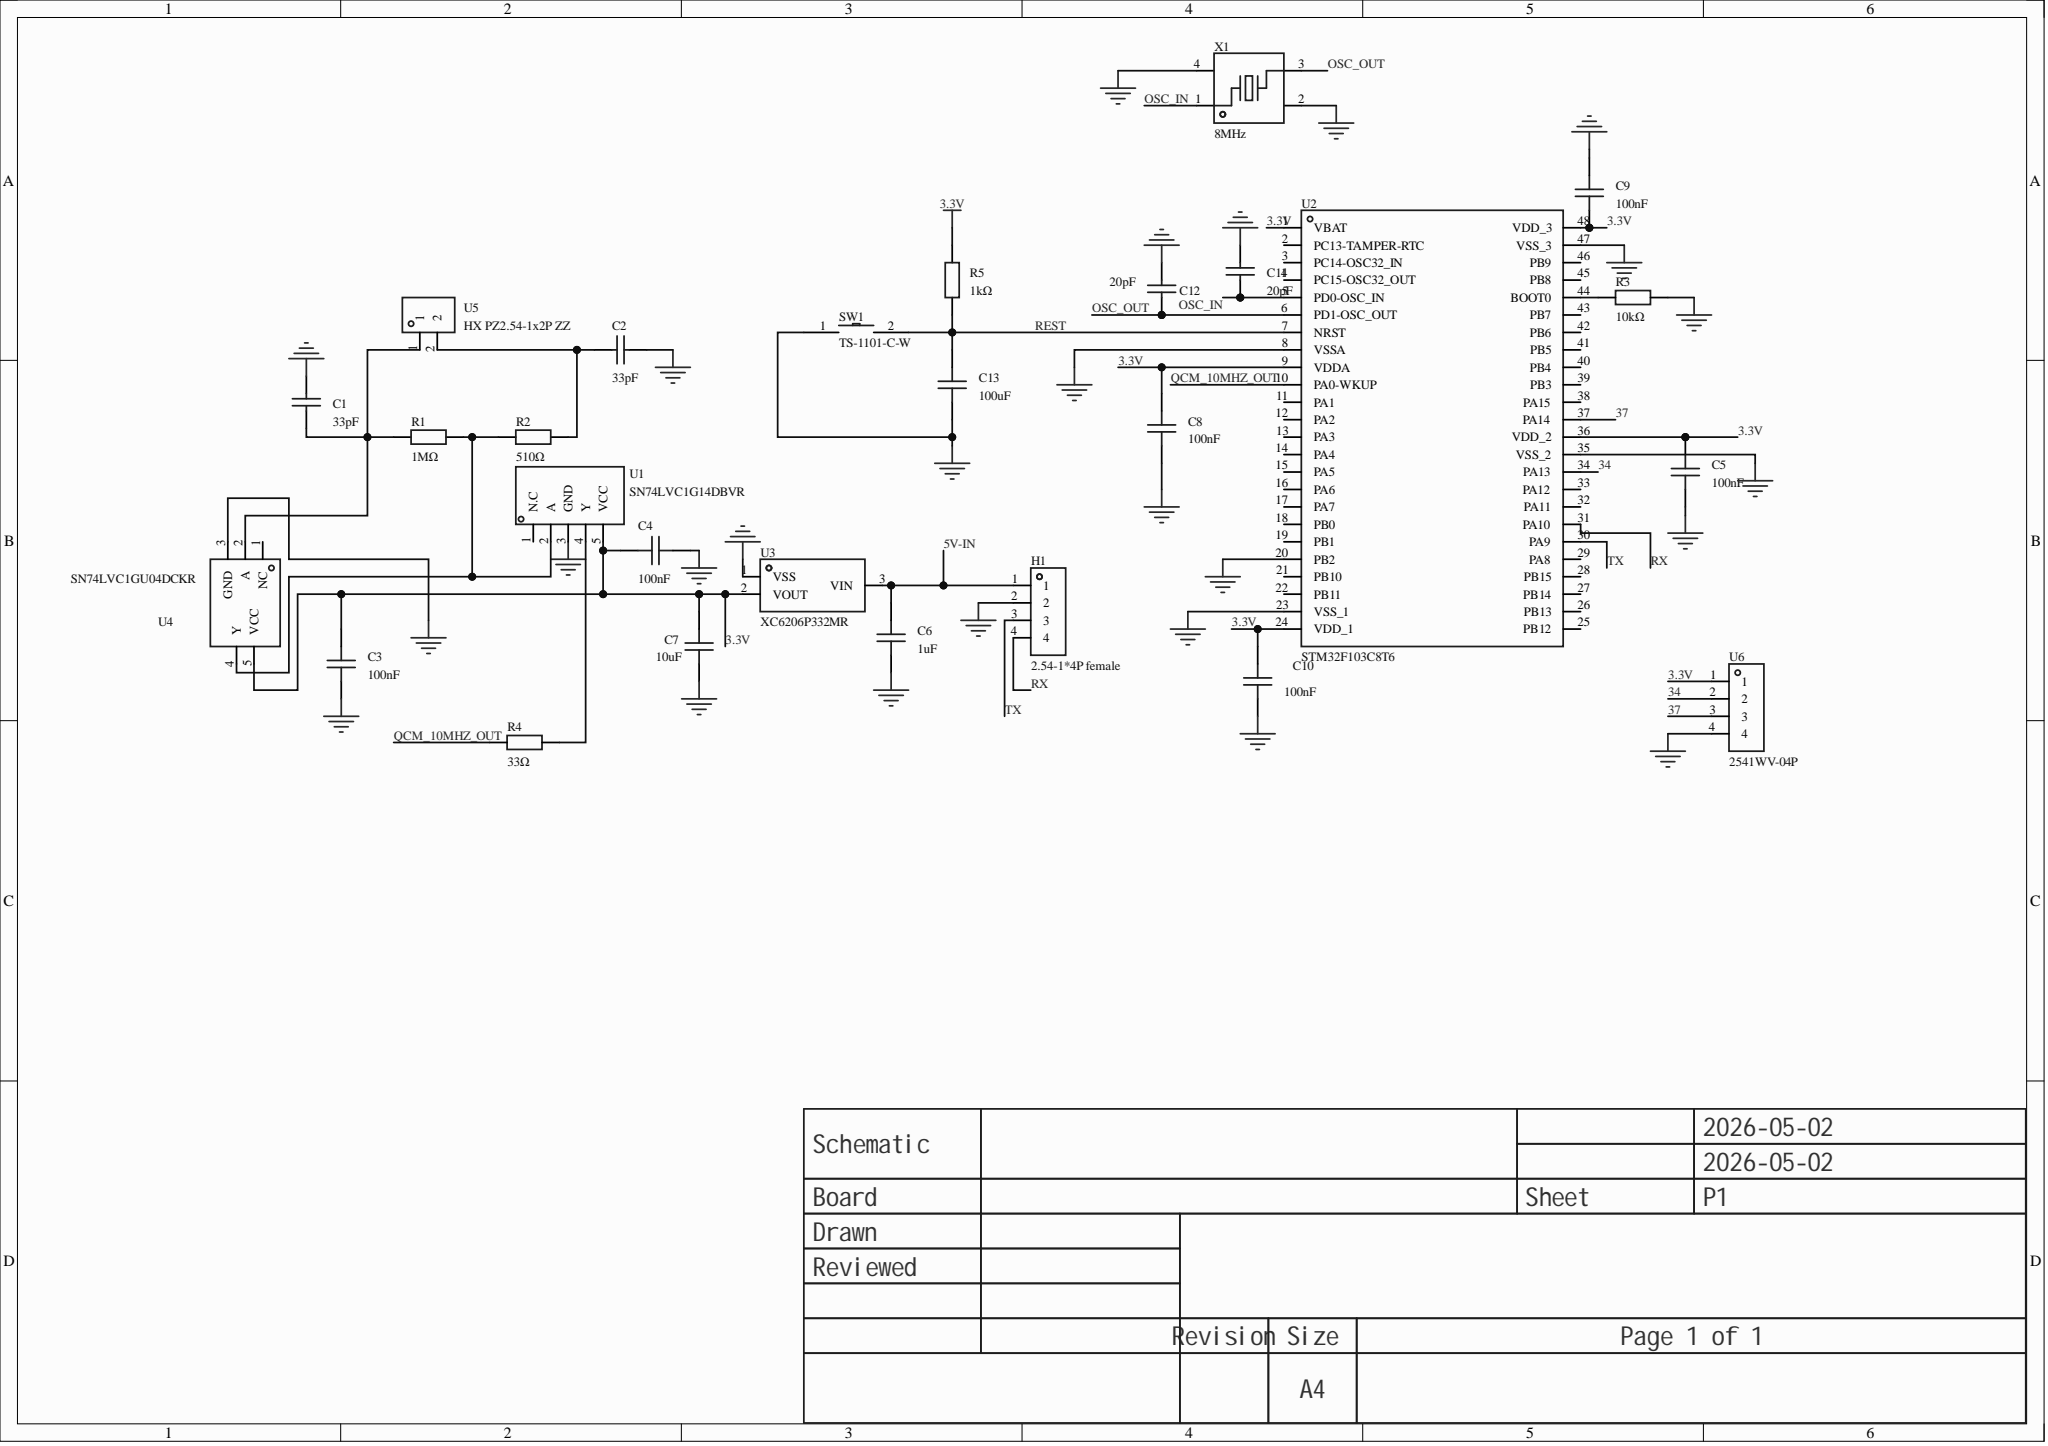Circuit board | Altium Designer | 27 parts | 16 nets
Bill of materials:
Comment,Description,Designator,Footprint,LibRef,Quantity
"33pF","Capacitance:33pF;Tolerance:±5%;Rated voltage:50V;Temperature coefficient:C0G;","C1, C2","C0603","CL10C330JB8NNNC","2"
"100nF","Capacitance:100nF;Tolerance:±10%;Rated voltage:50V;Temperature coefficient:X7R;","C3, C4, C5, C8, C9, C10","C0603","CGA0603X7R104K500JT","6"
"1uF","Capacitance:1uF;Tolerance:±10%;Rated voltage:50V;Temperature coefficient:X5R;","C6","C0603","CGA0603X5R105K500JT","1"
"10uF","Capacitance:1uF;Tolerance:±10%;Rated voltage:50V;Temperature coefficient:X5R;","C7","C0603","CGA0603X5R105K500JT","1"
"20pF","Capacitance:20pF;Tolerance:±5%;Rated voltage:50V;Temperature coefficient:C0G;","C11, C12","C0603","CL10C200JB8NNNC","2"
"100uF","Capacitance:100uF;Tolerance:±20%;Rated voltage:10V;Dielectric (temperature coefficient):X5R;","C13","C1206","HGC1206R5107M100NSPJ","1"
"2.54-1*4P female","Socket structure:1x4P;Pitch:2.54mm;Row spacing:-;Round/square hole:square hole;Mounting:through-hole;Rows:single row;Total holes:4P;Rated current:3A;Rated voltage:-;Socket direction:top;Plastic height:-;Contact material:Bronze;Contact plating:-;Operating temperature:-40℃~+105℃;","H1","HDR-TH_4P-P2.54-V-F","2.54-1*4P母","1"
"1MΩ","Resistor type:thick film;Resistance:1MΩ;Tolerance:±1%;Power:100mW;Max working voltage:75V;Temperature coefficient:±100ppm/?;","R1","R0603","0603WAF1004T5E","1"
"510Ω","Resistor type:thick film;Resistance:510Ω;Tolerance:±1%;Power:100mW;Working voltage:75V;Temperature coefficient:±100ppm/?;","R2","R0603","0603WAF5100T5E","1"
"10kΩ","","R3","R0603","Res_0603","1"
"33Ω","","R4","R0603","Res_0603","1"
"1kΩ","Resistor type:thick film;Resistance:1kΩ;Tolerance:±1%;Power:100mW;Max working voltage:75V;Temperature coefficient:±100ppm/?;","R5","R0603","RC0603FR-071KL","1"
"TS-1101-C-W","Circuit:SPST;Button shape:rectangular button;Actuating force:260gf;Mounting:surface mount;Switch length:6mm;Switch width:3.6mm;Switch height:2.5mm;Bracket:none;Contact current:50mA;Rated voltage (AC):-;Rated voltage (DC):12V;Rated power:-;Insulation resistance:-;Lamp:none;Mechanical life:5万 cycles;","SW1","SW-SMD_L6.0-W3.3-LS8.0","TS-1101-C-W","1"
"SN74LVC1G14DBVR","Input type:Schmitt trigger;Operating voltage:1.65V~5.5V;Quiescent current (Iq):10uA;Channels:1;Propagation delay (tpd):6.5ns@2.5V,50pF;","U1","SOT-23-5_L3.0-W1.7-P0.95-LS2.8-BR","SN74LVC1G14DBVR","1"
"STM32F103C8T6","CPU core:ARM-M3;Max CPU frequency:72MHz;Application field:-;","U2","LQFP-48_L7.0-W7.0-P0.50-LS9.0-BL","STM32F103C8T6","1"
"XC6206P332MR","Output type:fixed;Operating voltage:8V;Output voltage:3.3V;Output current:250mA;Ripple rejection (PSRR):40dB@(1kHz);Output polarity:positive;","U3","SOT-23-3_L3.0-W1.7-P0.95-LS2.9-BR","XC6206P332MR_C347376","1"
"SN74LVC1GU04DCKR","Input type:-;Operating voltage:1.65V~5.5V;Quiescent current (Iq):10uA;Channels:1;Propagation delay (tpd):3.5ns@5V,50pF;","U4","SC-70-5_L2.1-W1.3-P0.65-LS2.1-BL","SN74LVC1GU04DCKR","1"
"HX PZ2.54-1x2P ZZ","Pin structure:1x2P;Pitch:2.54mm;Row spacing:-;Round/square pin:square pin;Mounting:through-hole;Rows:single row;Total pins:2P;Rated current:3A;Rated voltage:1kV;Mating pin length:6mm;Plastic height:2.5mm;Termination pin length:3mm;Contact material:Brass;Contact plating:Gold;Operating temperature:-40℃~+105℃;Color:black;","U5","HDR-TH_2P-P2.54-V-M-3","HX PZ2.54-1x2P ZZ","1"
"2541WV-04P","Pin structure:1x4P;Pitch:2.54mm;Row spacing:-;Round/square pin:square pin;Mounting:through-hole;Rows:single row;Total pins:4P;Rated current:3A;Mating pin length:6mm;Plastic height:2.54mm;Termination pin length:3mm;Contact material:Brass;Contact plating:Gold;Operating temperature:-55℃~+105℃;","U6","HDR-TH_4P-P2.54-V-M-1","2541WV-04P","1"
"8MHz","Crystal type:SMD crystal;Frequency:8MHz;Tolerance at room temperature:±10ppm;Load capacitance:20pF;Frequency stability:±20ppm;","X1","CRYSTAL-SMD_4P-L3.2-W2.5-BL","X32258MSB4SI","1"
Netlist (Protel format):
[
C1
C0603
33pF



]
[
C2
C0603
33pF



]
[
C3
C0603
100nF



]
[
C4
C0603
100nF



]
[
C5
C0603
100nF



]
[
C6
C0603
1uF



]
[
C7
C0603
10uF



]
[
C8
C0603
100nF



]
[
C9
C0603
100nF



]
[
C10
C0603
100nF



]
[
C11
C0603
20pF



]
[
C12
C0603
20pF



]
[
C13
C1206
100uF



]
[
H1
HDR-TH_4P-P2.54-V-F
2.54-1*4P female



]
[
R1
R0603
1MΩ



]
[
R2
R0603
510Ω



]
[
R3
R0603
10kΩ



]
[
R4
R0603
33Ω



]
[
R5
R0603
1kΩ



]
[
SW1
SW-SMD_L6.0-W3.3-LS8.0
TS-1101-C-W



]
[
U1
SOT-23-5_L3.0-W1.7-P0.95-LS2.8-BR
SN74LVC1G14DBVR



]
[
U2
LQFP-48_L7.0-W7.0-P0.50-LS9.0-BL
STM32F103C8T6



]
[
U3
SOT-23-3_L3.0-W1.7-P0.95-LS2.9-BR
XC6206P332MR



]
[
U4
SC-70-5_L2.1-W1.3-P0.65-LS2.1-BL
SN74LVC1GU04DCKR



]
[
U5
HDR-TH_2P-P2.54-V-M-3
HX PZ2.54-1x2P ZZ



]
[
U6
HDR-TH_4P-P2.54-V-M-1
2541WV-04P



]
[
X1
CRYSTAL-SMD_4P-L3.2-W2.5-BL
8MHz



]
(
TX
H1-3
U2-30
)
(
RX
H1-4
U2-31
)
(
REST
C13-2
R5-1
SW1-2
U2-7
)
(
QCM_10MHZ_OUT
R4-1
U2-10
)
(
OSC_OUT
C12-1
U2-6
X1-3
)
(
OSC_IN
C11-1
U2-5
X1-1
)
(
NetR4_2
R4-2
U1-4
)
(
NetR3_1
R3-1
U2-44
)
(
NetR1_2
R1-2
R2-1
U1-2
U4-4
)
(
NetC2_1
C2-1
R2-2
U5-2
)
(
NetC1_1
C1-1
R1-1
U4-2
U5-1
)
(
GND
C1-2
C2-2
C3-1
C4-2
C5-1
C6-1
C7-1
C8-1
C9-2
C10-1
C11-2
C12-2
C13-1
H1-2
R3-2
SW1-1
U1-3
U2-8
U2-20
U2-23
U2-35
U2-47
U3-1
U4-3
U6-4
X1-2
X1-4
)
(
37
U2-37
U6-3
)
(
34
U2-34
U6-2
)
(
5V-IN
C6-2
H1-1
U3-3
)
(
3.3V
C3-2
C4-1
C5-2
C7-2
C8-2
C9-1
C10-2
R5-2
U1-5
U2-1
U2-9
U2-24
U2-36
U2-48
U3-2
U4-5
U6-1
)